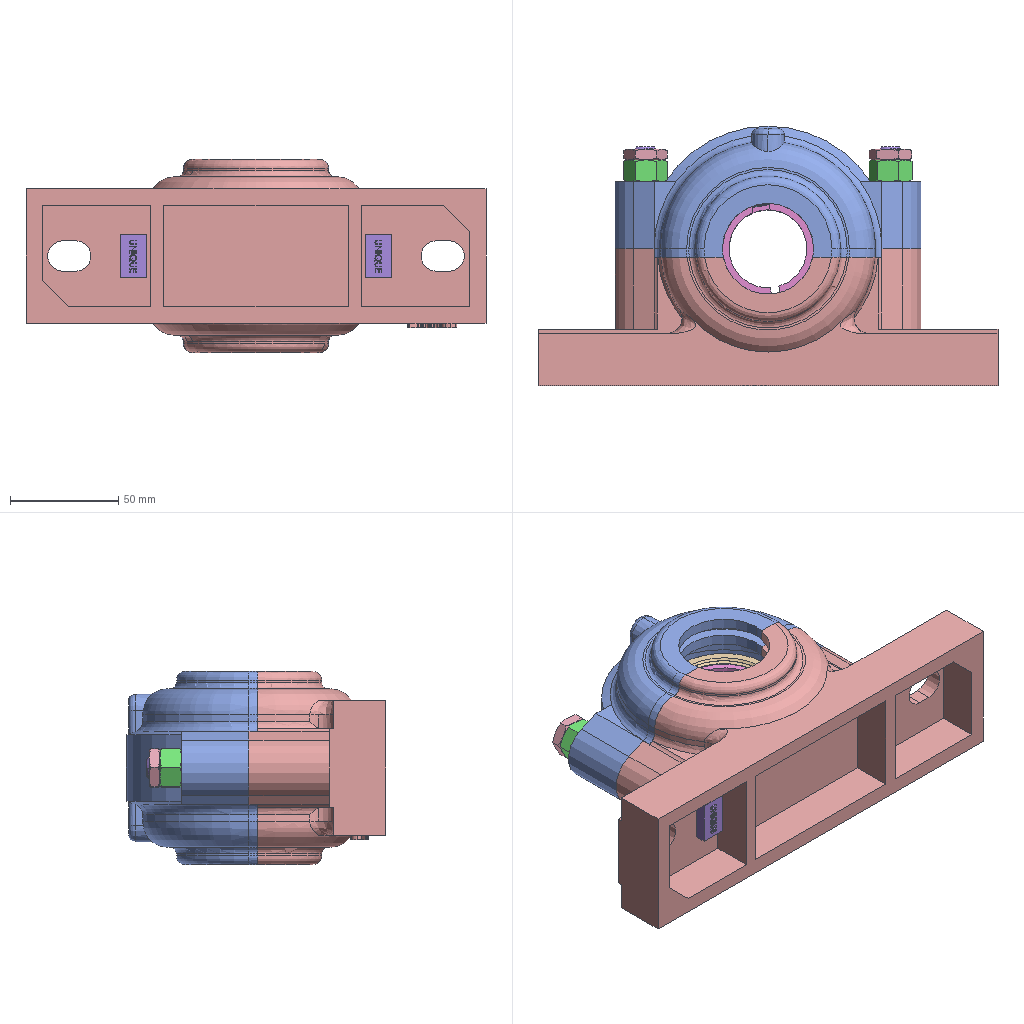Assembly | SolidWorks | 14 different items | 17 placed | box 212 x 120 x 89 mm
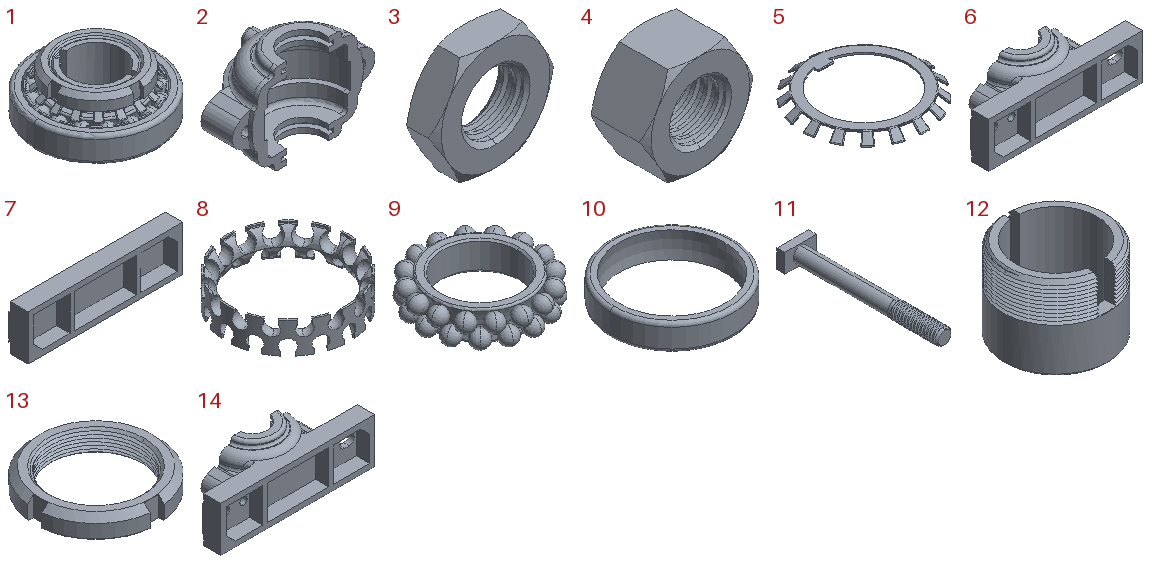Parts list (item | name | quantity | size | volume | features):
1 | (subassembly) | x1 | 85 x 85 x 37.81 mm | 92659 mm3 | -
2 | - | x1 | 141 x 60.5 x 89 mm | 190832 mm3 | features ICE 1, MirrorPattern 1, SplitBody 1
3 | - | x2 | 20 x 5 x 17.321 mm | 912.864 mm3 | features ICE 2, Chamfer 1, CombineBodies 1, Extrusion 1, MoveCopyBody 1, Stock 1
4 | - | x2 | 20 x 10 x 17.321 mm | 1854 mm3 | features ICE 2, Chamfer 1, CombineBodies 1, Extrusion 1, MoveCopyBody 1, Stock 1
5 | - | x1 | 65.578 x 65.38 x 4.578 mm | 1295 mm3 | features Fillet 3, ICE 2, CirPattern 1, Revolution 1
6 | - | x1 | 212 x 63 x 89 mm | 296687 mm3 | features ICE 6, MirrorPattern 2, VarFillet 2, CombineBodies 1, MoveCopyBody 1, RevCut 1, Revolution 1, Stock 1
7 | - | x1 | 212 x 26 x 62 mm | 172526 mm3 | features ICE 2, Extrusion 1, Rib 1, Shell 1
8 | - | x1 | 71 x 71 x 18 mm | 5623 mm3 | features CirPattern 2, ICE 2, CombineBodies 1, Extrusion 1, MoveCopyBody 1, RevCut 1, Revolution 1, Stock 1
9 | - | x1 | 74.417 x 74.417 x 18 mm | 31009 mm3 | features Chamfer 2, CirPattern 2, Revolution 2, Extrusion 1, Fillet 1, ICE 1, RevCut 1
10 | - | x1 | 85 x 85 x 18 mm | 23565 mm3 | features Extrusion 1, Fillet 1, RevCut 1
11 | - | x2 | 20 x 97 x 12 mm | 7646 mm3 | features ICE 2, Chamfer 1, Emboss 1, Extrusion 1, Helix 1, SweepCut 1
12 | - | x1 | 46 x 45.913 x 36 mm | 20268 mm3 | features Chamfer 2, ICE 2, Extrusion 1, Helix 1, SweepCut 1
13 | - | x1 | 59.59 x 59.59 x 10 mm | 10905 mm3 | features Chamfer 4, Helix 2, CirPattern 1, Extrusion 1, ICE 1, SweepCut 1
14 | - | x1 | 212 x 63 x 89 mm | 297133 mm3 | features ICE 8, MirrorPattern 3, VarFillet 2, CombineBodies 1, MoveCopyBody 1, RevCut 1, Revolution 1, Stock 1
Mates (type | each side: item.copy, entity, surface, feature):
Concentric | 14.1 face cylinder Cut-Extrude5 | 2.1 face cylinder Stock-Cap-1 | 2 times
Coincident | 14.1 face plane Cut-Extrude6 | 2.1 face plane Stock-Cap-1
Concentric | 10.1 face cylinder Boss-Extrude1 | 9.1 face cylinder Cut-Extrude1
Coincident | 10.1 face plane Boss-Extrude1 | 9.1 face plane Boss-Extrude1
Concentric | 10.1 face cylinder Boss-Extrude1 | 8.1 face cylinder Revolve1
Coincident | 10.1 face plane Boss-Extrude1 | 8.1 face plane Revolve1
Concentric | 9.1 face cylinder Cut-Extrude1 | 12.1 face cylinder Boss-Extrude1
DistanceDim | 12.1 face plane Boss-Extrude1 | 9.1 face plane Boss-Extrude1
Coincident | 9.1 plane | 12.1 plane
Coincident | 9.1 plane | 8.1 plane
Coincident | 12.1 face plane Cut-Extrude2 | 5.1 face plane Boss-Extrude1
Concentric | 12.1 face cylinder Boss-Extrude1 | 5.1 face cylinder Revolve1
Concentric | 12.1 face cylinder Boss-Extrude1 | 13.1 face cylinder Boss-Extrude1 | 2 times
Screw | 12.1 face cylinder Boss-Extrude1 | 13.1 face cylinder Boss-Extrude1
Concentric | 14.1 face cylinder Revolve1 | 10.1 face cylinder Boss-Extrude1
Concentric | 2.1 face cylinder Stock-Cap-1 | 11.1 face cylinder Boss-Extrude2
Parallel | 14.1 face plane Base2 | 11.1 face plane Boss-Extrude1
Coincident | 14.1 face plane Base2 | 11.1 face plane Boss-Extrude1
Concentric | 14.1 face cylinder Cut-Extrude5 | 11.2 face cylinder Boss-Extrude2
Parallel | 14.1 face plane Base2 | 11.2 face plane Boss-Extrude1
Coincident | 14.1 face plane Base2 | 11.2 face plane Boss-Extrude1
Concentric | 11.2 edge | 4.1 edge
Screw | 11.2 face cylinder Boss-Extrude3 | 4.1 face cylinder Combine1
Concentric | 11.2 face cylinder Boss-Extrude3 | 3.1 face cylinder Combine1
Screw | 11.2 face cylinder Boss-Extrude3 | 3.1 face cylinder Combine1
Concentric | 11.1 face cylinder Boss-Extrude3 | 4.2 face cylinder Combine1
Screw | 11.1 face cylinder Boss-Extrude3 | 4.2 face cylinder Boss-Extrude1
Concentric | 11.1 face cylinder Boss-Extrude3 | 3.2 face cylinder Combine1
Screw | 11.1 face cylinder Boss-Extrude3 | 3.2 face cylinder Combine1